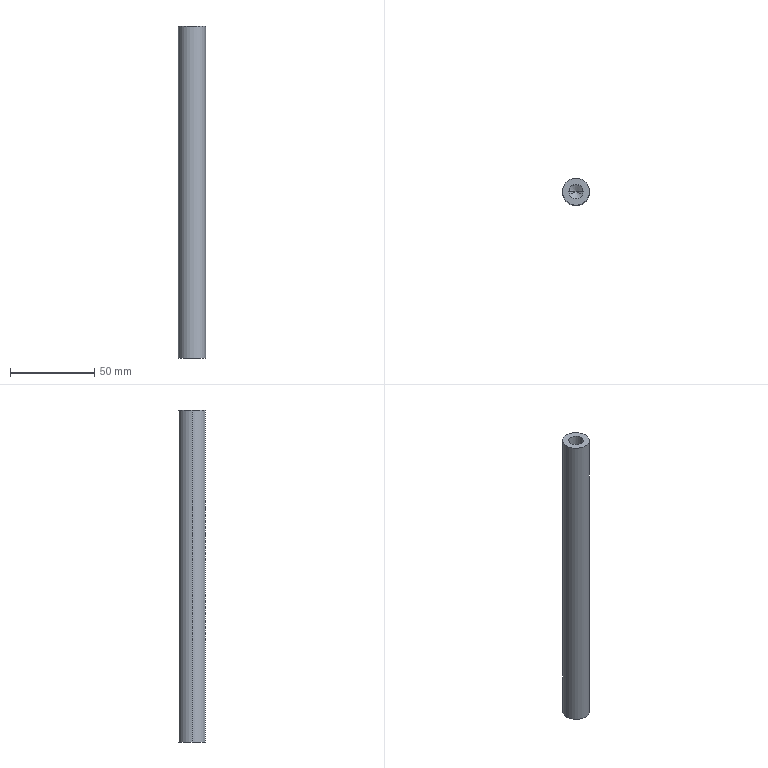Part | STEP file | B1-022 | 1 solid | 12 faces | box 16 x 16 x 196.5 mm | volume 37823 mm3 | cylinder 6 | cone 4 | plane 2 | commonest cylinder face diameters 8.5 x4 16 x2
STEP:
#1=CARTESIAN_POINT('',(0.,0.,0.));
#2=DIRECTION('',(0.,0.,1.));
#3=DIRECTION('',(1.,0.,0.));
#4=AXIS2_PLACEMENT_3D('',#1,#2,#3);
#5=CARTESIAN_POINT('',(4.25,0.,84.25));
#6=VERTEX_POINT('',#5);
#7=CARTESIAN_POINT('',(4.25,0.,98.25));
#8=VERTEX_POINT('',#7);
#9=CARTESIAN_POINT('',(4.25,0.,98.25));
#10=DIRECTION('',(0.,0.,1.));
#11=VECTOR('',#10,1.);
#12=LINE('',#9,#11);
#13=CARTESIAN_POINT('',(0.,0.,98.25));
#14=DIRECTION('',(0.,0.,1.));
#15=DIRECTION('',(1.,0.,0.));
#16=AXIS2_PLACEMENT_3D('',#13,#14,#15);
#17=CYLINDRICAL_SURFACE('',#16,4.25);
#18=CARTESIAN_POINT('',(6.283,0.));
#19=DIRECTION('',(0.,1.));
#20=VECTOR('',#19,1.);
#21=LINE('',#18,#20);
#22=(GEOMETRIC_REPRESENTATION_CONTEXT(2)PARAMETRIC_REPRESENTATION_CONTEXT()REPRESENTATION_CONTEXT('',''));
#23=DEFINITIONAL_REPRESENTATION('',(#21),#22);
#24=PCURVE('',#17,#23);
#25=CARTESIAN_POINT('',(0.,0.,98.25));
#26=DIRECTION('',(0.,0.,1.));
#27=DIRECTION('',(1.,0.,0.));
#28=AXIS2_PLACEMENT_3D('',#25,#26,#27);
#29=CYLINDRICAL_SURFACE('',#28,4.25);
#30=CARTESIAN_POINT('',(0.,0.));
#31=DIRECTION('',(0.,1.));
#32=VECTOR('',#31,1.);
#33=LINE('',#30,#32);
#34=(GEOMETRIC_REPRESENTATION_CONTEXT(2)PARAMETRIC_REPRESENTATION_CONTEXT()REPRESENTATION_CONTEXT('',''));
#35=DEFINITIONAL_REPRESENTATION('',(#33),#34);
#36=PCURVE('',#29,#35);
#37=SURFACE_CURVE('',#12,(#24,#36),.PCURVE_S1.);
#38=EDGE_CURVE('',#6,#8,#37,.T.);
#39=ORIENTED_EDGE('',*,*,#38,.T.);
#40=CARTESIAN_POINT('',(-4.25,0.,98.25));
#41=VERTEX_POINT('',#40);
#42=CARTESIAN_POINT('',(0.,0.,98.25));
#43=DIRECTION('',(0.,0.,1.));
#44=DIRECTION('',(1.,0.,0.));
#45=AXIS2_PLACEMENT_3D('',#42,#43,#44);
#46=CIRCLE('',#45,4.25);
#47=CARTESIAN_POINT('',(0.,0.));
#48=DIRECTION('',(1.,0.));
#49=VECTOR('',#48,1.);
#50=LINE('',#47,#49);
#51=(GEOMETRIC_REPRESENTATION_CONTEXT(2)PARAMETRIC_REPRESENTATION_CONTEXT()REPRESENTATION_CONTEXT('',''));
#52=DEFINITIONAL_REPRESENTATION('',(#50),#51);
#53=PCURVE('',#17,#52);
#54=CARTESIAN_POINT('',(0.,0.,98.25));
#55=DIRECTION('',(0.,0.,1.));
#56=DIRECTION('',(1.,0.,0.));
#57=AXIS2_PLACEMENT_3D('',#54,#55,#56);
#58=PLANE('',#57);
#59=CARTESIAN_POINT('',(0.,0.));
#60=DIRECTION('',(1.,0.));
#61=AXIS2_PLACEMENT_2D('',#59,#60);
#62=CIRCLE('',#61,4.25);
#63=(GEOMETRIC_REPRESENTATION_CONTEXT(2)PARAMETRIC_REPRESENTATION_CONTEXT()REPRESENTATION_CONTEXT('',''));
#64=DEFINITIONAL_REPRESENTATION('',(#62),#63);
#65=PCURVE('',#58,#64);
#66=SURFACE_CURVE('',#46,(#53,#65),.PCURVE_S1.);
#67=EDGE_CURVE('',#41,#8,#66,.T.);
#68=ORIENTED_EDGE('',*,*,#67,.F.);
#69=CARTESIAN_POINT('',(-4.25,0.,84.25));
#70=VERTEX_POINT('',#69);
#71=CARTESIAN_POINT('',(-4.25,0.,98.25));
#72=DIRECTION('',(0.,0.,1.));
#73=VECTOR('',#72,1.);
#74=LINE('',#71,#73);
#75=CARTESIAN_POINT('',(3.142,0.));
#76=DIRECTION('',(0.,1.));
#77=VECTOR('',#76,1.);
#78=LINE('',#75,#77);
#79=(GEOMETRIC_REPRESENTATION_CONTEXT(2)PARAMETRIC_REPRESENTATION_CONTEXT()REPRESENTATION_CONTEXT('',''));
#80=DEFINITIONAL_REPRESENTATION('',(#78),#79);
#81=PCURVE('',#17,#80);
#82=CARTESIAN_POINT('',(3.142,0.));
#83=DIRECTION('',(0.,1.));
#84=VECTOR('',#83,1.);
#85=LINE('',#82,#84);
#86=(GEOMETRIC_REPRESENTATION_CONTEXT(2)PARAMETRIC_REPRESENTATION_CONTEXT()REPRESENTATION_CONTEXT('',''));
#87=DEFINITIONAL_REPRESENTATION('',(#85),#86);
#88=PCURVE('',#29,#87);
#89=SURFACE_CURVE('',#74,(#81,#88),.PCURVE_S1.);
#90=EDGE_CURVE('',#70,#41,#89,.T.);
#91=ORIENTED_EDGE('',*,*,#90,.F.);
#92=CARTESIAN_POINT('',(0.,0.,84.25));
#93=DIRECTION('',(0.,0.,1.));
#94=DIRECTION('',(1.,0.,0.));
#95=AXIS2_PLACEMENT_3D('',#92,#93,#94);
#96=CIRCLE('',#95,4.25);
#97=CARTESIAN_POINT('',(0.,-14.));
#98=DIRECTION('',(1.,0.));
#99=VECTOR('',#98,1.);
#100=LINE('',#97,#99);
#101=(GEOMETRIC_REPRESENTATION_CONTEXT(2)PARAMETRIC_REPRESENTATION_CONTEXT()REPRESENTATION_CONTEXT('',''));
#102=DEFINITIONAL_REPRESENTATION('',(#100),#101);
#103=PCURVE('',#17,#102);
#104=CARTESIAN_POINT('',(0.,0.,84.25));
#105=DIRECTION('',(0.,0.,1.));
#106=DIRECTION('',(1.,0.,0.));
#107=AXIS2_PLACEMENT_3D('',#104,#105,#106);
#108=CONICAL_SURFACE('',#107,4.25,1.03);
#109=CARTESIAN_POINT('',(0.,0.));
#110=DIRECTION('',(1.,0.));
#111=VECTOR('',#110,1.);
#112=LINE('',#109,#111);
#113=(GEOMETRIC_REPRESENTATION_CONTEXT(2)PARAMETRIC_REPRESENTATION_CONTEXT()REPRESENTATION_CONTEXT('',''));
#114=DEFINITIONAL_REPRESENTATION('',(#112),#113);
#115=PCURVE('',#108,#114);
#116=SURFACE_CURVE('',#96,(#103,#115),.PCURVE_S1.);
#117=EDGE_CURVE('',#70,#6,#116,.T.);
#118=ORIENTED_EDGE('',*,*,#117,.T.);
#119=EDGE_LOOP('',(#39,#68,#91,#118));
#120=FACE_BOUND('',#119,.F.);
#121=ADVANCED_FACE('',(#120),#17,.F.);
#122=ORIENTED_EDGE('',*,*,#117,.F.);
#123=CARTESIAN_POINT('',(0.,0.,81.696));
#124=VERTEX_POINT('',#123);
#125=CARTESIAN_POINT('',(-4.25,0.,84.25));
#126=DIRECTION('',(-0.8572,0.,0.515));
#127=VECTOR('',#126,1.);
#128=LINE('',#125,#127);
#129=CARTESIAN_POINT('',(3.142,0.));
#130=DIRECTION('',(0.,1.));
#131=VECTOR('',#130,1.);
#132=LINE('',#129,#131);
#133=(GEOMETRIC_REPRESENTATION_CONTEXT(2)PARAMETRIC_REPRESENTATION_CONTEXT()REPRESENTATION_CONTEXT('',''));
#134=DEFINITIONAL_REPRESENTATION('',(#132),#133);
#135=PCURVE('',#108,#134);
#136=CARTESIAN_POINT('',(0.,0.,84.25));
#137=DIRECTION('',(0.,0.,1.));
#138=DIRECTION('',(1.,0.,0.));
#139=AXIS2_PLACEMENT_3D('',#136,#137,#138);
#140=CONICAL_SURFACE('',#139,4.25,1.03);
#141=CARTESIAN_POINT('',(3.142,0.));
#142=DIRECTION('',(0.,1.));
#143=VECTOR('',#142,1.);
#144=LINE('',#141,#143);
#145=(GEOMETRIC_REPRESENTATION_CONTEXT(2)PARAMETRIC_REPRESENTATION_CONTEXT()REPRESENTATION_CONTEXT('',''));
#146=DEFINITIONAL_REPRESENTATION('',(#144),#145);
#147=PCURVE('',#140,#146);
#148=SURFACE_CURVE('',#128,(#135,#147),.PCURVE_S1.);
#149=EDGE_CURVE('',#124,#70,#148,.T.);
#150=ORIENTED_EDGE('',*,*,#149,.F.);
#151=CARTESIAN_POINT('',(4.25,0.,84.25));
#152=DIRECTION('',(0.8572,0.,0.515));
#153=VECTOR('',#152,1.);
#154=LINE('',#151,#153);
#155=CARTESIAN_POINT('',(6.283,-2.554));
#156=CARTESIAN_POINT('',(6.283,-2.515));
#157=CARTESIAN_POINT('',(6.283,-2.438));
#158=CARTESIAN_POINT('',(6.283,-2.322));
#159=CARTESIAN_POINT('',(6.283,-2.205));
#160=CARTESIAN_POINT('',(6.283,-2.089));
#161=CARTESIAN_POINT('',(6.283,-1.973));
#162=CARTESIAN_POINT('',(6.283,-1.857));
#163=CARTESIAN_POINT('',(6.283,-1.741));
#164=CARTESIAN_POINT('',(6.283,-1.625));
#165=CARTESIAN_POINT('',(6.283,-1.509));
#166=CARTESIAN_POINT('',(6.283,-1.393));
#167=CARTESIAN_POINT('',(6.283,-1.277));
#168=CARTESIAN_POINT('',(6.283,-1.161));
#169=CARTESIAN_POINT('',(6.283,-1.045));
#170=CARTESIAN_POINT('',(6.283,-0.9286));
#171=CARTESIAN_POINT('',(6.283,-0.8125));
#172=CARTESIAN_POINT('',(6.283,-0.6965));
#173=CARTESIAN_POINT('',(6.283,-0.5804));
#174=CARTESIAN_POINT('',(6.283,-0.4643));
#175=CARTESIAN_POINT('',(6.283,-0.3482));
#176=CARTESIAN_POINT('',(6.283,-0.2322));
#177=CARTESIAN_POINT('',(6.283,-0.1161));
#178=CARTESIAN_POINT('',(6.283,-0.03869));
#179=CARTESIAN_POINT('',(6.283,0.));
#180=B_SPLINE_CURVE_WITH_KNOTS('',3,(#155,#156,#157,#158,#159,#160,#161,#162,#163,#164,#165,#166,#167,#168,#169,#170,#171,#172,#173,#174,#175,#176,#177,#178,#179),.UNSPECIFIED.,.F.,.F.,(4,1,1,1,1,1,1,1,1,1,1,1,1,1,1,1,1,1,1,1,1,1,4),(-4.958,-4.733,-4.507,-4.282,-4.057,-3.831,-3.606,-3.381,-3.155,-2.93,-2.704,-2.479,-2.254,-2.028,-1.803,-1.578,-1.352,-1.127,-0.9015,-0.6761,-0.4507,-0.2254,0.),.QUASI_UNIFORM_KNOTS.);
#181=(GEOMETRIC_REPRESENTATION_CONTEXT(2)PARAMETRIC_REPRESENTATION_CONTEXT()REPRESENTATION_CONTEXT('',''));
#182=DEFINITIONAL_REPRESENTATION('',(#180),#181);
#183=PCURVE('',#108,#182);
#184=CARTESIAN_POINT('',(0.,-2.554));
#185=CARTESIAN_POINT('',(0.,-2.515));
#186=CARTESIAN_POINT('',(0.,-2.438));
#187=CARTESIAN_POINT('',(0.,-2.322));
#188=CARTESIAN_POINT('',(0.,-2.205));
#189=CARTESIAN_POINT('',(0.,-2.089));
#190=CARTESIAN_POINT('',(0.,-1.973));
#191=CARTESIAN_POINT('',(0.,-1.857));
#192=CARTESIAN_POINT('',(0.,-1.741));
#193=CARTESIAN_POINT('',(0.,-1.625));
#194=CARTESIAN_POINT('',(0.,-1.509));
#195=CARTESIAN_POINT('',(0.,-1.393));
#196=CARTESIAN_POINT('',(0.,-1.277));
#197=CARTESIAN_POINT('',(0.,-1.161));
#198=CARTESIAN_POINT('',(0.,-1.045));
#199=CARTESIAN_POINT('',(0.,-0.9286));
#200=CARTESIAN_POINT('',(0.,-0.8125));
#201=CARTESIAN_POINT('',(0.,-0.6965));
#202=CARTESIAN_POINT('',(0.,-0.5804));
#203=CARTESIAN_POINT('',(0.,-0.4643));
#204=CARTESIAN_POINT('',(0.,-0.3482));
#205=CARTESIAN_POINT('',(0.,-0.2322));
#206=CARTESIAN_POINT('',(0.,-0.1161));
#207=CARTESIAN_POINT('',(0.,-0.03869));
#208=CARTESIAN_POINT('',(0.,0.));
#209=B_SPLINE_CURVE_WITH_KNOTS('',3,(#184,#185,#186,#187,#188,#189,#190,#191,#192,#193,#194,#195,#196,#197,#198,#199,#200,#201,#202,#203,#204,#205,#206,#207,#208),.UNSPECIFIED.,.F.,.F.,(4,1,1,1,1,1,1,1,1,1,1,1,1,1,1,1,1,1,1,1,1,1,4),(-4.958,-4.733,-4.507,-4.282,-4.057,-3.831,-3.606,-3.381,-3.155,-2.93,-2.704,-2.479,-2.254,-2.028,-1.803,-1.578,-1.352,-1.127,-0.9015,-0.6761,-0.4507,-0.2254,0.),.QUASI_UNIFORM_KNOTS.);
#210=(GEOMETRIC_REPRESENTATION_CONTEXT(2)PARAMETRIC_REPRESENTATION_CONTEXT()REPRESENTATION_CONTEXT('',''));
#211=DEFINITIONAL_REPRESENTATION('',(#209),#210);
#212=PCURVE('',#140,#211);
#213=SURFACE_CURVE('',#154,(#183,#212),.PCURVE_S1.);
#214=EDGE_CURVE('',#124,#6,#213,.T.);
#215=ORIENTED_EDGE('',*,*,#214,.T.);
#216=EDGE_LOOP('',(#122,#150,#215));
#217=FACE_BOUND('',#216,.F.);
#218=ADVANCED_FACE('',(#217),#108,.F.);
#219=CARTESIAN_POINT('',(-4.25,0.,-84.25));
#220=VERTEX_POINT('',#219);
#221=CARTESIAN_POINT('',(-4.25,0.,-98.25));
#222=VERTEX_POINT('',#221);
#223=CARTESIAN_POINT('',(-4.25,0.,-98.25));
#224=DIRECTION('',(0.,0.,-1.));
#225=VECTOR('',#224,1.);
#226=LINE('',#223,#225);
#227=CARTESIAN_POINT('',(0.,0.,-98.25));
#228=DIRECTION('',(0.,0.,-1.));
#229=DIRECTION('',(-1.,0.,0.));
#230=AXIS2_PLACEMENT_3D('',#227,#228,#229);
#231=CYLINDRICAL_SURFACE('',#230,4.25);
#232=CARTESIAN_POINT('',(6.283,0.));
#233=DIRECTION('',(0.,1.));
#234=VECTOR('',#233,1.);
#235=LINE('',#232,#234);
#236=(GEOMETRIC_REPRESENTATION_CONTEXT(2)PARAMETRIC_REPRESENTATION_CONTEXT()REPRESENTATION_CONTEXT('',''));
#237=DEFINITIONAL_REPRESENTATION('',(#235),#236);
#238=PCURVE('',#231,#237);
#239=CARTESIAN_POINT('',(0.,0.,-98.25));
#240=DIRECTION('',(0.,0.,-1.));
#241=DIRECTION('',(-1.,0.,0.));
#242=AXIS2_PLACEMENT_3D('',#239,#240,#241);
#243=CYLINDRICAL_SURFACE('',#242,4.25);
#244=CARTESIAN_POINT('',(0.,0.));
#245=DIRECTION('',(0.,1.));
#246=VECTOR('',#245,1.);
#247=LINE('',#244,#246);
#248=(GEOMETRIC_REPRESENTATION_CONTEXT(2)PARAMETRIC_REPRESENTATION_CONTEXT()REPRESENTATION_CONTEXT('',''));
#249=DEFINITIONAL_REPRESENTATION('',(#247),#248);
#250=PCURVE('',#243,#249);
#251=SURFACE_CURVE('',#226,(#238,#250),.PCURVE_S1.);
#252=EDGE_CURVE('',#220,#222,#251,.T.);
#253=ORIENTED_EDGE('',*,*,#252,.T.);
#254=CARTESIAN_POINT('',(4.25,0.,-98.25));
#255=VERTEX_POINT('',#254);
#256=CARTESIAN_POINT('',(0.,0.,-98.25));
#257=DIRECTION('',(0.,0.,-1.));
#258=DIRECTION('',(-1.,0.,0.));
#259=AXIS2_PLACEMENT_3D('',#256,#257,#258);
#260=CIRCLE('',#259,4.25);
#261=CARTESIAN_POINT('',(0.,0.));
#262=DIRECTION('',(1.,0.));
#263=VECTOR('',#262,1.);
#264=LINE('',#261,#263);
#265=(GEOMETRIC_REPRESENTATION_CONTEXT(2)PARAMETRIC_REPRESENTATION_CONTEXT()REPRESENTATION_CONTEXT('',''));
#266=DEFINITIONAL_REPRESENTATION('',(#264),#265);
#267=PCURVE('',#231,#266);
#268=CARTESIAN_POINT('',(0.,0.,-98.25));
#269=DIRECTION('',(0.,0.,1.));
#270=DIRECTION('',(1.,0.,0.));
#271=AXIS2_PLACEMENT_3D('',#268,#269,#270);
#272=PLANE('',#271);
#273=CARTESIAN_POINT('',(-4.25,0.));
#274=CARTESIAN_POINT('',(-4.25,7.361));
#275=CARTESIAN_POINT('',(2.125,3.681));
#276=CARTESIAN_POINT('',(8.5,0.));
#277=CARTESIAN_POINT('',(2.125,-3.681));
#278=CARTESIAN_POINT('',(-4.25,-7.361));
#279=CARTESIAN_POINT('',(-4.25,0.));
#280=(BOUNDED_CURVE()B_SPLINE_CURVE(2,(#273,#274,#275,#276,#277,#278,#279),.UNSPECIFIED.,.T.,.F.)B_SPLINE_CURVE_WITH_KNOTS((1,2,2,2,2,1),(-2.094,0.,2.094,4.189,6.283,8.378),.UNSPECIFIED.)CURVE()GEOMETRIC_REPRESENTATION_ITEM()RATIONAL_B_SPLINE_CURVE((1.,0.5,1.,0.5,1.,0.5,1.))REPRESENTATION_ITEM(''));
#281=(GEOMETRIC_REPRESENTATION_CONTEXT(2)PARAMETRIC_REPRESENTATION_CONTEXT()REPRESENTATION_CONTEXT('',''));
#282=DEFINITIONAL_REPRESENTATION('',(#280),#281);
#283=PCURVE('',#272,#282);
#284=SURFACE_CURVE('',#260,(#267,#283),.PCURVE_S1.);
#285=EDGE_CURVE('',#255,#222,#284,.T.);
#286=ORIENTED_EDGE('',*,*,#285,.F.);
#287=CARTESIAN_POINT('',(4.25,0.,-84.25));
#288=VERTEX_POINT('',#287);
#289=CARTESIAN_POINT('',(4.25,0.,-98.25));
#290=DIRECTION('',(0.,0.,-1.));
#291=VECTOR('',#290,1.);
#292=LINE('',#289,#291);
#293=CARTESIAN_POINT('',(3.142,0.));
#294=DIRECTION('',(0.,1.));
#295=VECTOR('',#294,1.);
#296=LINE('',#293,#295);
#297=(GEOMETRIC_REPRESENTATION_CONTEXT(2)PARAMETRIC_REPRESENTATION_CONTEXT()REPRESENTATION_CONTEXT('',''));
#298=DEFINITIONAL_REPRESENTATION('',(#296),#297);
#299=PCURVE('',#231,#298);
#300=CARTESIAN_POINT('',(3.142,0.));
#301=DIRECTION('',(0.,1.));
#302=VECTOR('',#301,1.);
#303=LINE('',#300,#302);
#304=(GEOMETRIC_REPRESENTATION_CONTEXT(2)PARAMETRIC_REPRESENTATION_CONTEXT()REPRESENTATION_CONTEXT('',''));
#305=DEFINITIONAL_REPRESENTATION('',(#303),#304);
#306=PCURVE('',#243,#305);
#307=SURFACE_CURVE('',#292,(#299,#306),.PCURVE_S1.);
#308=EDGE_CURVE('',#288,#255,#307,.T.);
#309=ORIENTED_EDGE('',*,*,#308,.F.);
#310=CARTESIAN_POINT('',(0.,0.,-84.25));
#311=DIRECTION('',(0.,0.,-1.));
#312=DIRECTION('',(-1.,0.,0.));
#313=AXIS2_PLACEMENT_3D('',#310,#311,#312);
#314=CIRCLE('',#313,4.25);
#315=CARTESIAN_POINT('',(0.,-14.));
#316=DIRECTION('',(1.,0.));
#317=VECTOR('',#316,1.);
#318=LINE('',#315,#317);
#319=(GEOMETRIC_REPRESENTATION_CONTEXT(2)PARAMETRIC_REPRESENTATION_CONTEXT()REPRESENTATION_CONTEXT('',''));
#320=DEFINITIONAL_REPRESENTATION('',(#318),#319);
#321=PCURVE('',#231,#320);
#322=CARTESIAN_POINT('',(0.,0.,-84.25));
#323=DIRECTION('',(0.,0.,-1.));
#324=DIRECTION('',(-1.,0.,0.));
#325=AXIS2_PLACEMENT_3D('',#322,#323,#324);
#326=CONICAL_SURFACE('',#325,4.25,1.03);
#327=CARTESIAN_POINT('',(0.,0.));
#328=DIRECTION('',(1.,0.));
#329=VECTOR('',#328,1.);
#330=LINE('',#327,#329);
#331=(GEOMETRIC_REPRESENTATION_CONTEXT(2)PARAMETRIC_REPRESENTATION_CONTEXT()REPRESENTATION_CONTEXT('',''));
#332=DEFINITIONAL_REPRESENTATION('',(#330),#331);
#333=PCURVE('',#326,#332);
#334=SURFACE_CURVE('',#314,(#321,#333),.PCURVE_S1.);
#335=EDGE_CURVE('',#288,#220,#334,.T.);
#336=ORIENTED_EDGE('',*,*,#335,.T.);
#337=EDGE_LOOP('',(#253,#286,#309,#336));
#338=FACE_BOUND('',#337,.F.);
#339=ADVANCED_FACE('',(#338),#231,.F.);
#340=ORIENTED_EDGE('',*,*,#335,.F.);
#341=CARTESIAN_POINT('',(0.,0.,-81.696));
#342=VERTEX_POINT('',#341);
#343=CARTESIAN_POINT('',(4.25,0.,-84.25));
#344=DIRECTION('',(0.8572,0.,-0.515));
#345=VECTOR('',#344,1.);
#346=LINE('',#343,#345);
#347=CARTESIAN_POINT('',(3.142,-2.554));
#348=CARTESIAN_POINT('',(3.142,-2.515));
#349=CARTESIAN_POINT('',(3.142,-2.438));
#350=CARTESIAN_POINT('',(3.142,-2.322));
#351=CARTESIAN_POINT('',(3.142,-2.205));
#352=CARTESIAN_POINT('',(3.142,-2.089));
#353=CARTESIAN_POINT('',(3.142,-1.973));
#354=CARTESIAN_POINT('',(3.142,-1.857));
#355=CARTESIAN_POINT('',(3.142,-1.741));
#356=CARTESIAN_POINT('',(3.142,-1.625));
#357=CARTESIAN_POINT('',(3.142,-1.509));
#358=CARTESIAN_POINT('',(3.142,-1.393));
#359=CARTESIAN_POINT('',(3.142,-1.277));
#360=CARTESIAN_POINT('',(3.142,-1.161));
#361=CARTESIAN_POINT('',(3.142,-1.045));
#362=CARTESIAN_POINT('',(3.142,-0.9286));
#363=CARTESIAN_POINT('',(3.142,-0.8125));
#364=CARTESIAN_POINT('',(3.142,-0.6965));
#365=CARTESIAN_POINT('',(3.142,-0.5804));
#366=CARTESIAN_POINT('',(3.142,-0.4643));
#367=CARTESIAN_POINT('',(3.142,-0.3482));
#368=CARTESIAN_POINT('',(3.142,-0.2322));
#369=CARTESIAN_POINT('',(3.142,-0.1161));
#370=CARTESIAN_POINT('',(3.142,-0.03869));
#371=CARTESIAN_POINT('',(3.142,0.));
#372=B_SPLINE_CURVE_WITH_KNOTS('',3,(#347,#348,#349,#350,#351,#352,#353,#354,#355,#356,#357,#358,#359,#360,#361,#362,#363,#364,#365,#366,#367,#368,#369,#370,#371),.UNSPECIFIED.,.F.,.F.,(4,1,1,1,1,1,1,1,1,1,1,1,1,1,1,1,1,1,1,1,1,1,4),(-4.958,-4.733,-4.507,-4.282,-4.057,-3.831,-3.606,-3.381,-3.155,-2.93,-2.704,-2.479,-2.254,-2.028,-1.803,-1.578,-1.352,-1.127,-0.9015,-0.6761,-0.4507,-0.2254,0.),.QUASI_UNIFORM_KNOTS.);
#373=(GEOMETRIC_REPRESENTATION_CONTEXT(2)PARAMETRIC_REPRESENTATION_CONTEXT()REPRESENTATION_CONTEXT('',''));
#374=DEFINITIONAL_REPRESENTATION('',(#372),#373);
#375=PCURVE('',#326,#374);
#376=CARTESIAN_POINT('',(0.,0.,-84.25));
#377=DIRECTION('',(0.,0.,-1.));
#378=DIRECTION('',(-1.,0.,0.));
#379=AXIS2_PLACEMENT_3D('',#376,#377,#378);
#380=CONICAL_SURFACE('',#379,4.25,1.03);
#381=CARTESIAN_POINT('',(3.142,-2.554));
#382=CARTESIAN_POINT('',(3.142,-2.515));
#383=CARTESIAN_POINT('',(3.142,-2.438));
#384=CARTESIAN_POINT('',(3.142,-2.322));
#385=CARTESIAN_POINT('',(3.142,-2.205));
#386=CARTESIAN_POINT('',(3.142,-2.089));
#387=CARTESIAN_POINT('',(3.142,-1.973));
#388=CARTESIAN_POINT('',(3.142,-1.857));
#389=CARTESIAN_POINT('',(3.142,-1.741));
#390=CARTESIAN_POINT('',(3.142,-1.625));
#391=CARTESIAN_POINT('',(3.142,-1.509));
#392=CARTESIAN_POINT('',(3.142,-1.393));
#393=CARTESIAN_POINT('',(3.142,-1.277));
#394=CARTESIAN_POINT('',(3.142,-1.161));
#395=CARTESIAN_POINT('',(3.142,-1.045));
#396=CARTESIAN_POINT('',(3.142,-0.9286));
#397=CARTESIAN_POINT('',(3.142,-0.8125));
#398=CARTESIAN_POINT('',(3.142,-0.6965));
#399=CARTESIAN_POINT('',(3.142,-0.5804));
#400=CARTESIAN_POINT('',(3.142,-0.4643));
#401=CARTESIAN_POINT('',(3.142,-0.3482));
#402=CARTESIAN_POINT('',(3.142,-0.2322));
#403=CARTESIAN_POINT('',(3.142,-0.1161));
#404=CARTESIAN_POINT('',(3.142,-0.03869));
#405=CARTESIAN_POINT('',(3.142,0.));
#406=B_SPLINE_CURVE_WITH_KNOTS('',3,(#381,#382,#383,#384,#385,#386,#387,#388,#389,#390,#391,#392,#393,#394,#395,#396,#397,#398,#399,#400,#401,#402,#403,#404,#405),.UNSPECIFIED.,.F.,.F.,(4,1,1,1,1,1,1,1,1,1,1,1,1,1,1,1,1,1,1,1,1,1,4),(-4.958,-4.733,-4.507,-4.282,-4.057,-3.831,-3.606,-3.381,-3.155,-2.93,-2.704,-2.479,-2.254,-2.028,-1.803,-1.578,-1.352,-1.127,-0.9015,-0.6761,-0.4507,-0.2254,0.),.QUASI_UNIFORM_KNOTS.);
#407=(GEOMETRIC_REPRESENTATION_CONTEXT(2)PARAMETRIC_REPRESENTATION_CONTEXT()REPRESENTATION_CONTEXT('',''));
#408=DEFINITIONAL_REPRESENTATION('',(#406),#407);
#409=PCURVE('',#380,#408);
#410=SURFACE_CURVE('',#346,(#375,#409),.PCURVE_S1.);
#411=EDGE_CURVE('',#342,#288,#410,.T.);
#412=ORIENTED_EDGE('',*,*,#411,.F.);
#413=CARTESIAN_POINT('',(-4.25,0.,-84.25));
#414=DIRECTION('',(-0.8572,0.,-0.515));
#415=VECTOR('',#414,1.);
#416=LINE('',#413,#415);
#417=CARTESIAN_POINT('',(6.283,0.));
#418=DIRECTION('',(0.,1.));
#419=VECTOR('',#418,1.);
#420=LINE('',#417,#419);
#421=(GEOMETRIC_REPRESENTATION_CONTEXT(2)PARAMETRIC_REPRESENTATION_CONTEXT()REPRESENTATION_CONTEXT('',''));
#422=DEFINITIONAL_REPRESENTATION('',(#420),#421);
#423=PCURVE('',#326,#422);
#424=CARTESIAN_POINT('',(0.,0.));
#425=DIRECTION('',(0.,1.));
#426=VECTOR('',#425,1.);
#427=LINE('',#424,#426);
#428=(GEOMETRIC_REPRESENTATION_CONTEXT(2)PARAMETRIC_REPRESENTATION_CONTEXT()REPRESENTATION_CONTEXT('',''));
#429=DEFINITIONAL_REPRESENTATION('',(#427),#428);
#430=PCURVE('',#380,#429);
#431=SURFACE_CURVE('',#416,(#423,#430),.PCURVE_S1.);
#432=EDGE_CURVE('',#342,#220,#431,.T.);
#433=ORIENTED_EDGE('',*,*,#432,.T.);
#434=EDGE_LOOP('',(#340,#412,#433));
#435=FACE_BOUND('',#434,.F.);
#436=ADVANCED_FACE('',(#435),#326,.F.);
#437=CARTESIAN_POINT('',(8.,0.,98.25));
#438=VERTEX_POINT('',#437);
#439=CARTESIAN_POINT('',(-8.,0.,98.25));
#440=VERTEX_POINT('',#439);
#441=CARTESIAN_POINT('',(0.,0.,98.25));
#442=DIRECTION('',(0.,0.,1.));
#443=DIRECTION('',(1.,0.,0.));
#444=AXIS2_PLACEMENT_3D('',#441,#442,#443);
#445=CIRCLE('',#444,8.);
#446=CARTESIAN_POINT('',(0.,0.,98.25));
#447=DIRECTION('',(0.,0.,-1.));
#448=DIRECTION('',(-1.,0.,0.));
#449=AXIS2_PLACEMENT_3D('',#446,#447,#448);
#450=CYLINDRICAL_SURFACE('',#449,8.);
#451=CARTESIAN_POINT('',(3.142,0.));
#452=DIRECTION('',(-1.,0.));
#453=VECTOR('',#452,1.);
#454=LINE('',#451,#453);
#455=(GEOMETRIC_REPRESENTATION_CONTEXT(2)PARAMETRIC_REPRESENTATION_CONTEXT()REPRESENTATION_CONTEXT('',''));
#456=DEFINITIONAL_REPRESENTATION('',(#454),#455);
#457=PCURVE('',#450,#456);
#458=CARTESIAN_POINT('',(0.,0.));
#459=DIRECTION('',(1.,0.));
#460=AXIS2_PLACEMENT_2D('',#458,#459);
#461=CIRCLE('',#460,8.);
#462=(GEOMETRIC_REPRESENTATION_CONTEXT(2)PARAMETRIC_REPRESENTATION_CONTEXT()REPRESENTATION_CONTEXT('',''));
#463=DEFINITIONAL_REPRESENTATION('',(#461),#462);
#464=PCURVE('',#58,#463);
#465=SURFACE_CURVE('',#445,(#457,#464),.PCURVE_S1.);
#466=EDGE_CURVE('',#438,#440,#465,.T.);
#467=ORIENTED_EDGE('',*,*,#466,.F.);
#468=CARTESIAN_POINT('',(8.,0.,-98.25));
#469=VERTEX_POINT('',#468);
#470=CARTESIAN_POINT('',(8.,0.,98.25));
#471=DIRECTION('',(0.,0.,-1.));
#472=VECTOR('',#471,1.);
#473=LINE('',#470,#472);
#474=CARTESIAN_POINT('',(3.142,0.));
#475=DIRECTION('',(0.,1.));
#476=VECTOR('',#475,1.);
#477=LINE('',#474,#476);
#478=(GEOMETRIC_REPRESENTATION_CONTEXT(2)PARAMETRIC_REPRESENTATION_CONTEXT()REPRESENTATION_CONTEXT('',''));
#479=DEFINITIONAL_REPRESENTATION('',(#477),#478);
#480=PCURVE('',#450,#479);
#481=CARTESIAN_POINT('',(0.,0.,98.25));
#482=DIRECTION('',(0.,0.,-1.));
#483=DIRECTION('',(-1.,0.,0.));
#484=AXIS2_PLACEMENT_3D('',#481,#482,#483);
#485=CYLINDRICAL_SURFACE('',#484,8.);
#486=CARTESIAN_POINT('',(3.142,0.));
#487=DIRECTION('',(0.,1.));
#488=VECTOR('',#487,1.);
#489=LINE('',#486,#488);
#490=(GEOMETRIC_REPRESENTATION_CONTEXT(2)PARAMETRIC_REPRESENTATION_CONTEXT()REPRESENTATION_CONTEXT('',''));
#491=DEFINITIONAL_REPRESENTATION('',(#489),#490);
#492=PCURVE('',#485,#491);
#493=SURFACE_CURVE('',#473,(#480,#492),.PCURVE_S1.);
#494=EDGE_CURVE('',#438,#469,#493,.T.);
#495=ORIENTED_EDGE('',*,*,#494,.T.);
#496=CARTESIAN_POINT('',(-8.,0.,-98.25));
#497=VERTEX_POINT('',#496);
#498=CARTESIAN_POINT('',(0.,0.,-98.25));
#499=DIRECTION('',(0.,0.,1.));
#500=DIRECTION('',(1.,0.,0.));
#501=AXIS2_PLACEMENT_3D('',#498,#499,#500);
#502=CIRCLE('',#501,8.);
#503=CARTESIAN_POINT('',(3.142,196.5));
#504=DIRECTION('',(-1.,0.));
#505=VECTOR('',#504,1.);
#506=LINE('',#503,#505);
#507=(GEOMETRIC_REPRESENTATION_CONTEXT(2)PARAMETRIC_REPRESENTATION_CONTEXT()REPRESENTATION_CONTEXT('',''));
#508=DEFINITIONAL_REPRESENTATION('',(#506),#507);
#509=PCURVE('',#450,#508);
#510=CARTESIAN_POINT('',(0.,0.));
#511=DIRECTION('',(1.,0.));
#512=AXIS2_PLACEMENT_2D('',#510,#511);
#513=CIRCLE('',#512,8.);
#514=(GEOMETRIC_REPRESENTATION_CONTEXT(2)PARAMETRIC_REPRESENTATION_CONTEXT()REPRESENTATION_CONTEXT('',''));
#515=DEFINITIONAL_REPRESENTATION('',(#513),#514);
#516=PCURVE('',#272,#515);
#517=SURFACE_CURVE('',#502,(#509,#516),.PCURVE_S1.);
#518=EDGE_CURVE('',#469,#497,#517,.T.);
#519=ORIENTED_EDGE('',*,*,#518,.T.);
#520=CARTESIAN_POINT('',(-8.,0.,98.25));
#521=DIRECTION('',(0.,0.,-1.));
#522=VECTOR('',#521,1.);
#523=LINE('',#520,#522);
#524=CARTESIAN_POINT('',(0.,0.));
#525=DIRECTION('',(0.,1.));
#526=VECTOR('',#525,1.);
#527=LINE('',#524,#526);
#528=(GEOMETRIC_REPRESENTATION_CONTEXT(2)PARAMETRIC_REPRESENTATION_CONTEXT()REPRESENTATION_CONTEXT('',''));
#529=DEFINITIONAL_REPRESENTATION('',(#527),#528);
#530=PCURVE('',#450,#529);
#531=CARTESIAN_POINT('',(6.283,0.));
#532=DIRECTION('',(0.,1.));
#533=VECTOR('',#532,1.);
#534=LINE('',#531,#533);
#535=(GEOMETRIC_REPRESENTATION_CONTEXT(2)PARAMETRIC_REPRESENTATION_CONTEXT()REPRESENTATION_CONTEXT('',''));
#536=DEFINITIONAL_REPRESENTATION('',(#534),#535);
#537=PCURVE('',#485,#536);
#538=SURFACE_CURVE('',#523,(#530,#537),.PCURVE_S1.);
#539=EDGE_CURVE('',#440,#497,#538,.T.);
#540=ORIENTED_EDGE('',*,*,#539,.F.);
#541=EDGE_LOOP('',(#467,#495,#519,#540));
#542=FACE_BOUND('',#541,.T.);
#543=ADVANCED_FACE('',(#542),#450,.T.);
#544=ORIENTED_EDGE('',*,*,#494,.F.);
#545=CARTESIAN_POINT('',(0.,0.,98.25));
#546=DIRECTION('',(0.,0.,1.));
#547=DIRECTION('',(1.,0.,0.));
#548=AXIS2_PLACEMENT_3D('',#545,#546,#547);
#549=CIRCLE('',#548,8.);
#550=CARTESIAN_POINT('',(9.425,0.));
#551=DIRECTION('',(-1.,0.));
#552=VECTOR('',#551,1.);
#553=LINE('',#550,#552);
#554=(GEOMETRIC_REPRESENTATION_CONTEXT(2)PARAMETRIC_REPRESENTATION_CONTEXT()REPRESENTATION_CONTEXT('',''));
#555=DEFINITIONAL_REPRESENTATION('',(#553),#554);
#556=PCURVE('',#485,#555);
#557=CARTESIAN_POINT('',(0.,0.));
#558=DIRECTION('',(1.,0.));
#559=AXIS2_PLACEMENT_2D('',#557,#558);
#560=CIRCLE('',#559,8.);
#561=(GEOMETRIC_REPRESENTATION_CONTEXT(2)PARAMETRIC_REPRESENTATION_CONTEXT()REPRESENTATION_CONTEXT('',''));
#562=DEFINITIONAL_REPRESENTATION('',(#560),#561);
#563=PCURVE('',#58,#562);
#564=SURFACE_CURVE('',#549,(#556,#563),.PCURVE_S1.);
#565=EDGE_CURVE('',#440,#438,#564,.T.);
#566=ORIENTED_EDGE('',*,*,#565,.F.);
#567=ORIENTED_EDGE('',*,*,#539,.T.);
#568=CARTESIAN_POINT('',(0.,0.,-98.25));
#569=DIRECTION('',(0.,0.,1.));
#570=DIRECTION('',(1.,0.,0.));
#571=AXIS2_PLACEMENT_3D('',#568,#569,#570);
#572=CIRCLE('',#571,8.);
#573=CARTESIAN_POINT('',(9.425,196.5));
#574=DIRECTION('',(-1.,0.));
#575=VECTOR('',#574,1.);
#576=LINE('',#573,#575);
#577=(GEOMETRIC_REPRESENTATION_CONTEXT(2)PARAMETRIC_REPRESENTATION_CONTEXT()REPRESENTATION_CONTEXT('',''));
#578=DEFINITIONAL_REPRESENTATION('',(#576),#577);
#579=PCURVE('',#485,#578);
#580=CARTESIAN_POINT('',(0.,0.));
#581=DIRECTION('',(1.,0.));
#582=AXIS2_PLACEMENT_2D('',#580,#581);
#583=CIRCLE('',#582,8.);
#584=(GEOMETRIC_REPRESENTATION_CONTEXT(2)PARAMETRIC_REPRESENTATION_CONTEXT()REPRESENTATION_CONTEXT('',''));
#585=DEFINITIONAL_REPRESENTATION('',(#583),#584);
#586=PCURVE('',#272,#585);
#587=SURFACE_CURVE('',#572,(#579,#586),.PCURVE_S1.);
#588=EDGE_CURVE('',#497,#469,#587,.T.);
#589=ORIENTED_EDGE('',*,*,#588,.T.);
#590=EDGE_LOOP('',(#544,#566,#567,#589));
#591=FACE_BOUND('',#590,.T.);
#592=ADVANCED_FACE('',(#591),#485,.T.);
#593=CARTESIAN_POINT('',(0.,0.,98.25));
#594=DIRECTION('',(0.,0.,1.));
#595=DIRECTION('',(1.,0.,0.));
#596=AXIS2_PLACEMENT_3D('',#593,#594,#595);
#597=CIRCLE('',#596,4.25);
#598=CARTESIAN_POINT('',(0.,0.));
#599=DIRECTION('',(1.,0.));
#600=AXIS2_PLACEMENT_2D('',#598,#599);
#601=CIRCLE('',#600,4.25);
#602=(GEOMETRIC_REPRESENTATION_CONTEXT(2)PARAMETRIC_REPRESENTATION_CONTEXT()REPRESENTATION_CONTEXT('',''));
#603=DEFINITIONAL_REPRESENTATION('',(#601),#602);
#604=PCURVE('',#58,#603);
#605=CARTESIAN_POINT('',(0.,0.));
#606=DIRECTION('',(1.,0.));
#607=VECTOR('',#606,1.);
#608=LINE('',#605,#607);
#609=(GEOMETRIC_REPRESENTATION_CONTEXT(2)PARAMETRIC_REPRESENTATION_CONTEXT()REPRESENTATION_CONTEXT('',''));
#610=DEFINITIONAL_REPRESENTATION('',(#608),#609);
#611=PCURVE('',#29,#610);
#612=SURFACE_CURVE('',#597,(#604,#611),.PCURVE_S1.);
#613=EDGE_CURVE('',#8,#41,#612,.T.);
#614=ORIENTED_EDGE('',*,*,#613,.F.);
#615=ORIENTED_EDGE('',*,*,#67,.F.);
#616=EDGE_LOOP('',(#614,#615));
#617=FACE_BOUND('',#616,.T.);
#618=ORIENTED_EDGE('',*,*,#565,.T.);
#619=ORIENTED_EDGE('',*,*,#466,.T.);
#620=EDGE_LOOP('',(#618,#619));
#621=FACE_BOUND('',#620,.T.);
#622=ADVANCED_FACE('',(#617,#621),#58,.T.);
#623=CARTESIAN_POINT('',(0.,0.,-98.25));
#624=DIRECTION('',(0.,0.,-1.));
#625=DIRECTION('',(-1.,0.,0.));
#626=AXIS2_PLACEMENT_3D('',#623,#624,#625);
#627=CIRCLE('',#626,4.25);
#628=CARTESIAN_POINT('',(-4.25,0.));
#629=CARTESIAN_POINT('',(-4.25,7.361));
#630=CARTESIAN_POINT('',(2.125,3.681));
#631=CARTESIAN_POINT('',(8.5,0.));
#632=CARTESIAN_POINT('',(2.125,-3.681));
#633=CARTESIAN_POINT('',(-4.25,-7.361));
#634=CARTESIAN_POINT('',(-4.25,0.));
#635=(BOUNDED_CURVE()B_SPLINE_CURVE(2,(#628,#629,#630,#631,#632,#633,#634),.UNSPECIFIED.,.T.,.F.)B_SPLINE_CURVE_WITH_KNOTS((1,2,2,2,2,1),(-2.094,0.,2.094,4.189,6.283,8.378),.UNSPECIFIED.)CURVE()GEOMETRIC_REPRESENTATION_ITEM()RATIONAL_B_SPLINE_CURVE((1.,0.5,1.,0.5,1.,0.5,1.))REPRESENTATION_ITEM(''));
#636=(GEOMETRIC_REPRESENTATION_CONTEXT(2)PARAMETRIC_REPRESENTATION_CONTEXT()REPRESENTATION_CONTEXT('',''));
#637=DEFINITIONAL_REPRESENTATION('',(#635),#636);
#638=PCURVE('',#272,#637);
#639=CARTESIAN_POINT('',(0.,0.));
#640=DIRECTION('',(1.,0.));
#641=VECTOR('',#640,1.);
#642=LINE('',#639,#641);
#643=(GEOMETRIC_REPRESENTATION_CONTEXT(2)PARAMETRIC_REPRESENTATION_CONTEXT()REPRESENTATION_CONTEXT('',''));
#644=DEFINITIONAL_REPRESENTATION('',(#642),#643);
#645=PCURVE('',#243,#644);
#646=SURFACE_CURVE('',#627,(#638,#645),.PCURVE_S1.);
#647=EDGE_CURVE('',#222,#255,#646,.T.);
#648=ORIENTED_EDGE('',*,*,#647,.F.);
#649=ORIENTED_EDGE('',*,*,#285,.F.);
#650=EDGE_LOOP('',(#648,#649));
#651=FACE_BOUND('',#650,.T.);
#652=ORIENTED_EDGE('',*,*,#588,.F.);
#653=ORIENTED_EDGE('',*,*,#518,.F.);
#654=EDGE_LOOP('',(#652,#653));
#655=FACE_BOUND('',#654,.T.);
#656=ADVANCED_FACE('',(#651,#655),#272,.F.);
#657=CARTESIAN_POINT('',(0.,0.,-84.25));
#658=DIRECTION('',(0.,0.,-1.));
#659=DIRECTION('',(-1.,0.,0.));
#660=AXIS2_PLACEMENT_3D('',#657,#658,#659);
#661=CIRCLE('',#660,4.25);
#662=CARTESIAN_POINT('',(0.,0.));
#663=DIRECTION('',(1.,0.));
#664=VECTOR('',#663,1.);
#665=LINE('',#662,#664);
#666=(GEOMETRIC_REPRESENTATION_CONTEXT(2)PARAMETRIC_REPRESENTATION_CONTEXT()REPRESENTATION_CONTEXT('',''));
#667=DEFINITIONAL_REPRESENTATION('',(#665),#666);
#668=PCURVE('',#380,#667);
#669=CARTESIAN_POINT('',(0.,-14.));
#670=DIRECTION('',(1.,0.));
#671=VECTOR('',#670,1.);
#672=LINE('',#669,#671);
#673=(GEOMETRIC_REPRESENTATION_CONTEXT(2)PARAMETRIC_REPRESENTATION_CONTEXT()REPRESENTATION_CONTEXT('',''));
#674=DEFINITIONAL_REPRESENTATION('',(#672),#673);
#675=PCURVE('',#243,#674);
#676=SURFACE_CURVE('',#661,(#668,#675),.PCURVE_S1.);
#677=EDGE_CURVE('',#220,#288,#676,.T.);
#678=ORIENTED_EDGE('',*,*,#677,.F.);
#679=ORIENTED_EDGE('',*,*,#432,.F.);
#680=ORIENTED_EDGE('',*,*,#411,.T.);
#681=EDGE_LOOP('',(#678,#679,#680));
#682=FACE_BOUND('',#681,.F.);
#683=ADVANCED_FACE('',(#682),#380,.F.);
#684=ORIENTED_EDGE('',*,*,#647,.F.);
#685=ORIENTED_EDGE('',*,*,#252,.F.);
#686=ORIENTED_EDGE('',*,*,#677,.T.);
#687=ORIENTED_EDGE('',*,*,#308,.T.);
#688=EDGE_LOOP('',(#684,#685,#686,#687));
#689=FACE_BOUND('',#688,.F.);
#690=ADVANCED_FACE('',(#689),#243,.F.);
#691=CARTESIAN_POINT('',(0.,0.,84.25));
#692=DIRECTION('',(0.,0.,1.));
#693=DIRECTION('',(1.,0.,0.));
#694=AXIS2_PLACEMENT_3D('',#691,#692,#693);
#695=CIRCLE('',#694,4.25);
#696=CARTESIAN_POINT('',(0.,0.));
#697=DIRECTION('',(1.,0.));
#698=VECTOR('',#697,1.);
#699=LINE('',#696,#698);
#700=(GEOMETRIC_REPRESENTATION_CONTEXT(2)PARAMETRIC_REPRESENTATION_CONTEXT()REPRESENTATION_CONTEXT('',''));
#701=DEFINITIONAL_REPRESENTATION('',(#699),#700);
#702=PCURVE('',#140,#701);
#703=CARTESIAN_POINT('',(0.,-14.));
#704=DIRECTION('',(1.,0.));
#705=VECTOR('',#704,1.);
#706=LINE('',#703,#705);
#707=(GEOMETRIC_REPRESENTATION_CONTEXT(2)PARAMETRIC_REPRESENTATION_CONTEXT()REPRESENTATION_CONTEXT('',''));
#708=DEFINITIONAL_REPRESENTATION('',(#706),#707);
#709=PCURVE('',#29,#708);
#710=SURFACE_CURVE('',#695,(#702,#709),.PCURVE_S1.);
#711=EDGE_CURVE('',#6,#70,#710,.T.);
#712=ORIENTED_EDGE('',*,*,#711,.F.);
#713=ORIENTED_EDGE('',*,*,#214,.F.);
#714=ORIENTED_EDGE('',*,*,#149,.T.);
#715=EDGE_LOOP('',(#712,#713,#714));
#716=FACE_BOUND('',#715,.F.);
#717=ADVANCED_FACE('',(#716),#140,.F.);
#718=ORIENTED_EDGE('',*,*,#613,.F.);
#719=ORIENTED_EDGE('',*,*,#38,.F.);
#720=ORIENTED_EDGE('',*,*,#711,.T.);
#721=ORIENTED_EDGE('',*,*,#90,.T.);
#722=EDGE_LOOP('',(#718,#719,#720,#721));
#723=FACE_BOUND('',#722,.F.);
#724=ADVANCED_FACE('',(#723),#29,.F.);
#725=CLOSED_SHELL('',(#121,#218,#339,#436,#543,#592,#622,#656,#683,#690,#717,#724));
#726=MANIFOLD_SOLID_BREP('',#725);
#727=(LENGTH_UNIT()NAMED_UNIT(*)SI_UNIT(.MILLI.,.METRE.));
#728=UNCERTAINTY_MEASURE_WITH_UNIT(LENGTH_MEASURE(0.0000001),#727,'','');
#729=(NAMED_UNIT(*)PLANE_ANGLE_UNIT()SI_UNIT($,.RADIAN.));
#730=(NAMED_UNIT(*)SI_UNIT($,.STERADIAN.)SOLID_ANGLE_UNIT());
#731=(GEOMETRIC_REPRESENTATION_CONTEXT(3)GLOBAL_UNCERTAINTY_ASSIGNED_CONTEXT((#728))GLOBAL_UNIT_ASSIGNED_CONTEXT((#727,#729,#730))REPRESENTATION_CONTEXT('',''));
#732=ADVANCED_BREP_SHAPE_REPRESENTATION('',(#4,#726),#731);